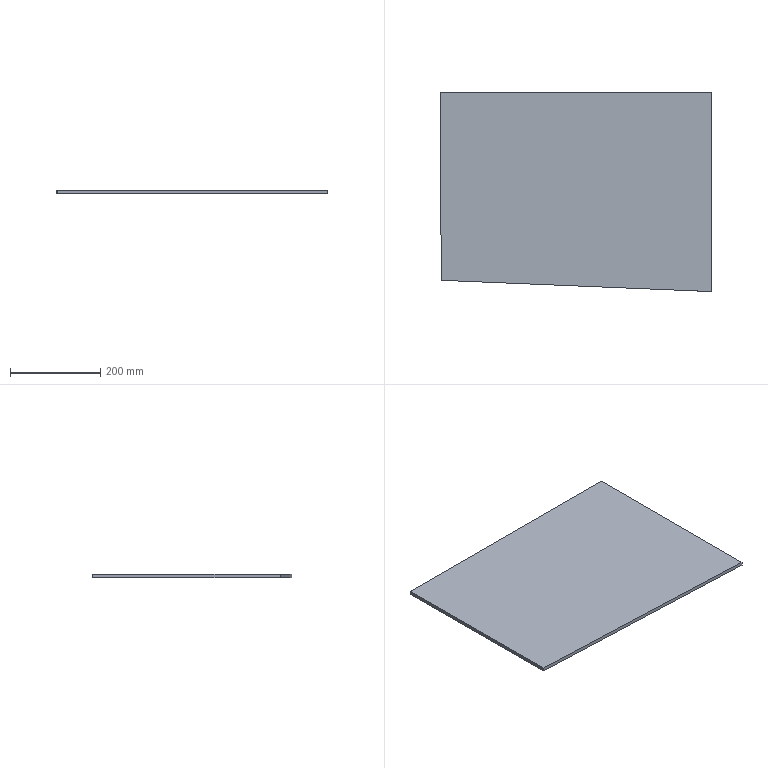Part | STEP file | 06-Middle plate | 1 solid | 6 faces | box 600 x 442 x 8 mm | volume 2060678 mm3 | plane 6
STEP:
#1=CARTESIAN_POINT('',(0.,0.,0.));
#2=DIRECTION('',(0.,0.,1.));
#3=DIRECTION('',(1.,0.,0.));
#4=AXIS2_PLACEMENT_3D('',#1,#2,#3);
#5=CARTESIAN_POINT('',(0.,0.,0.));
#6=VERTEX_POINT('',#5);
#7=CARTESIAN_POINT('',(0.5211,-417.,0.));
#8=VERTEX_POINT('',#7);
#9=CARTESIAN_POINT('',(0.,0.,0.));
#10=DIRECTION('',(0.00125,-1.,0.));
#11=VECTOR('',#10,1.);
#12=LINE('',#9,#11);
#13=CARTESIAN_POINT('',(0.,0.,8.));
#14=DIRECTION('',(1.,0.00125,0.));
#15=DIRECTION('',(-0.00125,1.,0.));
#16=AXIS2_PLACEMENT_3D('',#13,#14,#15);
#17=PLANE('',#16);
#18=CARTESIAN_POINT('',(0.,-8.));
#19=DIRECTION('',(-1.,0.));
#20=VECTOR('',#19,1.);
#21=LINE('',#18,#20);
#22=(GEOMETRIC_REPRESENTATION_CONTEXT(2)PARAMETRIC_REPRESENTATION_CONTEXT()REPRESENTATION_CONTEXT('',''));
#23=DEFINITIONAL_REPRESENTATION('',(#21),#22);
#24=PCURVE('',#17,#23);
#25=CARTESIAN_POINT('',(0.,0.,0.));
#26=DIRECTION('',(0.,0.,1.));
#27=DIRECTION('',(1.,0.,0.));
#28=AXIS2_PLACEMENT_3D('',#25,#26,#27);
#29=PLANE('',#28);
#30=CARTESIAN_POINT('',(0.,0.));
#31=DIRECTION('',(0.00125,-1.));
#32=VECTOR('',#31,1.);
#33=LINE('',#30,#32);
#34=(GEOMETRIC_REPRESENTATION_CONTEXT(2)PARAMETRIC_REPRESENTATION_CONTEXT()REPRESENTATION_CONTEXT('',''));
#35=DEFINITIONAL_REPRESENTATION('',(#33),#34);
#36=PCURVE('',#29,#35);
#37=SURFACE_CURVE('',#12,(#24,#36),.PCURVE_S1.);
#38=EDGE_CURVE('',#6,#8,#37,.T.);
#39=ORIENTED_EDGE('',*,*,#38,.T.);
#40=CARTESIAN_POINT('',(0.5211,-417.,8.));
#41=VERTEX_POINT('',#40);
#42=CARTESIAN_POINT('',(0.5211,-417.,8.));
#43=DIRECTION('',(0.,0.,-1.));
#44=VECTOR('',#43,1.);
#45=LINE('',#42,#44);
#46=CARTESIAN_POINT('',(-417.,0.));
#47=DIRECTION('',(0.,-1.));
#48=VECTOR('',#47,1.);
#49=LINE('',#46,#48);
#50=(GEOMETRIC_REPRESENTATION_CONTEXT(2)PARAMETRIC_REPRESENTATION_CONTEXT()REPRESENTATION_CONTEXT('',''));
#51=DEFINITIONAL_REPRESENTATION('',(#49),#50);
#52=PCURVE('',#17,#51);
#53=CARTESIAN_POINT('',(0.5211,-417.,8.));
#54=DIRECTION('',(0.04167,0.9991,0.));
#55=DIRECTION('',(-0.9991,0.04167,0.));
#56=AXIS2_PLACEMENT_3D('',#53,#54,#55);
#57=PLANE('',#56);
#58=CARTESIAN_POINT('',(0.,0.));
#59=DIRECTION('',(0.,-1.));
#60=VECTOR('',#59,1.);
#61=LINE('',#58,#60);
#62=(GEOMETRIC_REPRESENTATION_CONTEXT(2)PARAMETRIC_REPRESENTATION_CONTEXT()REPRESENTATION_CONTEXT('',''));
#63=DEFINITIONAL_REPRESENTATION('',(#61),#62);
#64=PCURVE('',#57,#63);
#65=SURFACE_CURVE('',#45,(#52,#64),.PCURVE_S1.);
#66=EDGE_CURVE('',#41,#8,#65,.T.);
#67=ORIENTED_EDGE('',*,*,#66,.F.);
#68=CARTESIAN_POINT('',(0.,0.,8.));
#69=VERTEX_POINT('',#68);
#70=CARTESIAN_POINT('',(0.,0.,8.));
#71=DIRECTION('',(0.00125,-1.,0.));
#72=VECTOR('',#71,1.);
#73=LINE('',#70,#72);
#74=CARTESIAN_POINT('',(0.,0.));
#75=DIRECTION('',(-1.,0.));
#76=VECTOR('',#75,1.);
#77=LINE('',#74,#76);
#78=(GEOMETRIC_REPRESENTATION_CONTEXT(2)PARAMETRIC_REPRESENTATION_CONTEXT()REPRESENTATION_CONTEXT('',''));
#79=DEFINITIONAL_REPRESENTATION('',(#77),#78);
#80=PCURVE('',#17,#79);
#81=CARTESIAN_POINT('',(0.,0.,8.));
#82=DIRECTION('',(0.,0.,1.));
#83=DIRECTION('',(1.,0.,0.));
#84=AXIS2_PLACEMENT_3D('',#81,#82,#83);
#85=PLANE('',#84);
#86=CARTESIAN_POINT('',(0.,0.));
#87=DIRECTION('',(0.00125,-1.));
#88=VECTOR('',#87,1.);
#89=LINE('',#86,#88);
#90=(GEOMETRIC_REPRESENTATION_CONTEXT(2)PARAMETRIC_REPRESENTATION_CONTEXT()REPRESENTATION_CONTEXT('',''));
#91=DEFINITIONAL_REPRESENTATION('',(#89),#90);
#92=PCURVE('',#85,#91);
#93=SURFACE_CURVE('',#73,(#80,#92),.PCURVE_S1.);
#94=EDGE_CURVE('',#69,#41,#93,.T.);
#95=ORIENTED_EDGE('',*,*,#94,.F.);
#96=CARTESIAN_POINT('',(0.,0.,8.));
#97=DIRECTION('',(0.,0.,-1.));
#98=VECTOR('',#97,1.);
#99=LINE('',#96,#98);
#100=CARTESIAN_POINT('',(0.,0.));
#101=DIRECTION('',(0.,-1.));
#102=VECTOR('',#101,1.);
#103=LINE('',#100,#102);
#104=(GEOMETRIC_REPRESENTATION_CONTEXT(2)PARAMETRIC_REPRESENTATION_CONTEXT()REPRESENTATION_CONTEXT('',''));
#105=DEFINITIONAL_REPRESENTATION('',(#103),#104);
#106=PCURVE('',#17,#105);
#107=CARTESIAN_POINT('',(0.,0.,8.));
#108=DIRECTION('',(0.,-1.,0.));
#109=DIRECTION('',(0.,0.,-1.));
#110=AXIS2_PLACEMENT_3D('',#107,#108,#109);
#111=PLANE('',#110);
#112=CARTESIAN_POINT('',(0.,0.));
#113=DIRECTION('',(1.,0.));
#114=VECTOR('',#113,1.);
#115=LINE('',#112,#114);
#116=(GEOMETRIC_REPRESENTATION_CONTEXT(2)PARAMETRIC_REPRESENTATION_CONTEXT()REPRESENTATION_CONTEXT('',''));
#117=DEFINITIONAL_REPRESENTATION('',(#115),#116);
#118=PCURVE('',#111,#117);
#119=SURFACE_CURVE('',#99,(#106,#118),.PCURVE_S1.);
#120=EDGE_CURVE('',#69,#6,#119,.T.);
#121=ORIENTED_EDGE('',*,*,#120,.T.);
#122=EDGE_LOOP('',(#39,#67,#95,#121));
#123=FACE_BOUND('',#122,.T.);
#124=ADVANCED_FACE('',(#123),#17,.F.);
#125=CARTESIAN_POINT('',(600.,-442.,0.));
#126=VERTEX_POINT('',#125);
#127=CARTESIAN_POINT('',(0.5211,-417.,0.));
#128=DIRECTION('',(0.9991,-0.04167,0.));
#129=VECTOR('',#128,1.);
#130=LINE('',#127,#129);
#131=CARTESIAN_POINT('',(0.,-8.));
#132=DIRECTION('',(-1.,0.));
#133=VECTOR('',#132,1.);
#134=LINE('',#131,#133);
#135=(GEOMETRIC_REPRESENTATION_CONTEXT(2)PARAMETRIC_REPRESENTATION_CONTEXT()REPRESENTATION_CONTEXT('',''));
#136=DEFINITIONAL_REPRESENTATION('',(#134),#135);
#137=PCURVE('',#57,#136);
#138=CARTESIAN_POINT('',(0.5211,-417.));
#139=DIRECTION('',(0.9991,-0.04167));
#140=VECTOR('',#139,1.);
#141=LINE('',#138,#140);
#142=(GEOMETRIC_REPRESENTATION_CONTEXT(2)PARAMETRIC_REPRESENTATION_CONTEXT()REPRESENTATION_CONTEXT('',''));
#143=DEFINITIONAL_REPRESENTATION('',(#141),#142);
#144=PCURVE('',#29,#143);
#145=SURFACE_CURVE('',#130,(#137,#144),.PCURVE_S1.);
#146=EDGE_CURVE('',#8,#126,#145,.T.);
#147=ORIENTED_EDGE('',*,*,#146,.T.);
#148=CARTESIAN_POINT('',(600.,-442.,8.));
#149=VERTEX_POINT('',#148);
#150=CARTESIAN_POINT('',(600.,-442.,8.));
#151=DIRECTION('',(0.,0.,-1.));
#152=VECTOR('',#151,1.);
#153=LINE('',#150,#152);
#154=CARTESIAN_POINT('',(-600.,0.));
#155=DIRECTION('',(0.,-1.));
#156=VECTOR('',#155,1.);
#157=LINE('',#154,#156);
#158=(GEOMETRIC_REPRESENTATION_CONTEXT(2)PARAMETRIC_REPRESENTATION_CONTEXT()REPRESENTATION_CONTEXT('',''));
#159=DEFINITIONAL_REPRESENTATION('',(#157),#158);
#160=PCURVE('',#57,#159);
#161=CARTESIAN_POINT('',(600.,0.,8.));
#162=DIRECTION('',(-1.,0.,0.));
#163=DIRECTION('',(0.,-1.,0.));
#164=AXIS2_PLACEMENT_3D('',#161,#162,#163);
#165=PLANE('',#164);
#166=CARTESIAN_POINT('',(442.,0.));
#167=DIRECTION('',(0.,-1.));
#168=VECTOR('',#167,1.);
#169=LINE('',#166,#168);
#170=(GEOMETRIC_REPRESENTATION_CONTEXT(2)PARAMETRIC_REPRESENTATION_CONTEXT()REPRESENTATION_CONTEXT('',''));
#171=DEFINITIONAL_REPRESENTATION('',(#169),#170);
#172=PCURVE('',#165,#171);
#173=SURFACE_CURVE('',#153,(#160,#172),.PCURVE_S1.);
#174=EDGE_CURVE('',#149,#126,#173,.T.);
#175=ORIENTED_EDGE('',*,*,#174,.F.);
#176=CARTESIAN_POINT('',(0.5211,-417.,8.));
#177=DIRECTION('',(0.9991,-0.04167,0.));
#178=VECTOR('',#177,1.);
#179=LINE('',#176,#178);
#180=CARTESIAN_POINT('',(0.,0.));
#181=DIRECTION('',(-1.,0.));
#182=VECTOR('',#181,1.);
#183=LINE('',#180,#182);
#184=(GEOMETRIC_REPRESENTATION_CONTEXT(2)PARAMETRIC_REPRESENTATION_CONTEXT()REPRESENTATION_CONTEXT('',''));
#185=DEFINITIONAL_REPRESENTATION('',(#183),#184);
#186=PCURVE('',#57,#185);
#187=CARTESIAN_POINT('',(0.5211,-417.));
#188=DIRECTION('',(0.9991,-0.04167));
#189=VECTOR('',#188,1.);
#190=LINE('',#187,#189);
#191=(GEOMETRIC_REPRESENTATION_CONTEXT(2)PARAMETRIC_REPRESENTATION_CONTEXT()REPRESENTATION_CONTEXT('',''));
#192=DEFINITIONAL_REPRESENTATION('',(#190),#191);
#193=PCURVE('',#85,#192);
#194=SURFACE_CURVE('',#179,(#186,#193),.PCURVE_S1.);
#195=EDGE_CURVE('',#41,#149,#194,.T.);
#196=ORIENTED_EDGE('',*,*,#195,.F.);
#197=ORIENTED_EDGE('',*,*,#66,.T.);
#198=EDGE_LOOP('',(#147,#175,#196,#197));
#199=FACE_BOUND('',#198,.T.);
#200=ADVANCED_FACE('',(#199),#57,.F.);
#201=CARTESIAN_POINT('',(600.,0.,0.));
#202=VERTEX_POINT('',#201);
#203=CARTESIAN_POINT('',(600.,0.,0.));
#204=DIRECTION('',(0.,1.,0.));
#205=VECTOR('',#204,1.);
#206=LINE('',#203,#205);
#207=CARTESIAN_POINT('',(0.,-8.));
#208=DIRECTION('',(-1.,0.));
#209=VECTOR('',#208,1.);
#210=LINE('',#207,#209);
#211=(GEOMETRIC_REPRESENTATION_CONTEXT(2)PARAMETRIC_REPRESENTATION_CONTEXT()REPRESENTATION_CONTEXT('',''));
#212=DEFINITIONAL_REPRESENTATION('',(#210),#211);
#213=PCURVE('',#165,#212);
#214=CARTESIAN_POINT('',(600.,0.));
#215=DIRECTION('',(0.,1.));
#216=VECTOR('',#215,1.);
#217=LINE('',#214,#216);
#218=(GEOMETRIC_REPRESENTATION_CONTEXT(2)PARAMETRIC_REPRESENTATION_CONTEXT()REPRESENTATION_CONTEXT('',''));
#219=DEFINITIONAL_REPRESENTATION('',(#217),#218);
#220=PCURVE('',#29,#219);
#221=SURFACE_CURVE('',#206,(#213,#220),.PCURVE_S1.);
#222=EDGE_CURVE('',#126,#202,#221,.T.);
#223=ORIENTED_EDGE('',*,*,#222,.T.);
#224=CARTESIAN_POINT('',(600.,0.,8.));
#225=VERTEX_POINT('',#224);
#226=CARTESIAN_POINT('',(600.,0.,8.));
#227=DIRECTION('',(0.,0.,-1.));
#228=VECTOR('',#227,1.);
#229=LINE('',#226,#228);
#230=CARTESIAN_POINT('',(0.,0.));
#231=DIRECTION('',(0.,-1.));
#232=VECTOR('',#231,1.);
#233=LINE('',#230,#232);
#234=(GEOMETRIC_REPRESENTATION_CONTEXT(2)PARAMETRIC_REPRESENTATION_CONTEXT()REPRESENTATION_CONTEXT('',''));
#235=DEFINITIONAL_REPRESENTATION('',(#233),#234);
#236=PCURVE('',#165,#235);
#237=CARTESIAN_POINT('',(0.,600.));
#238=DIRECTION('',(1.,0.));
#239=VECTOR('',#238,1.);
#240=LINE('',#237,#239);
#241=(GEOMETRIC_REPRESENTATION_CONTEXT(2)PARAMETRIC_REPRESENTATION_CONTEXT()REPRESENTATION_CONTEXT('',''));
#242=DEFINITIONAL_REPRESENTATION('',(#240),#241);
#243=PCURVE('',#111,#242);
#244=SURFACE_CURVE('',#229,(#236,#243),.PCURVE_S1.);
#245=EDGE_CURVE('',#225,#202,#244,.T.);
#246=ORIENTED_EDGE('',*,*,#245,.F.);
#247=CARTESIAN_POINT('',(600.,0.,8.));
#248=DIRECTION('',(0.,1.,0.));
#249=VECTOR('',#248,1.);
#250=LINE('',#247,#249);
#251=CARTESIAN_POINT('',(0.,0.));
#252=DIRECTION('',(-1.,0.));
#253=VECTOR('',#252,1.);
#254=LINE('',#251,#253);
#255=(GEOMETRIC_REPRESENTATION_CONTEXT(2)PARAMETRIC_REPRESENTATION_CONTEXT()REPRESENTATION_CONTEXT('',''));
#256=DEFINITIONAL_REPRESENTATION('',(#254),#255);
#257=PCURVE('',#165,#256);
#258=CARTESIAN_POINT('',(600.,0.));
#259=DIRECTION('',(0.,1.));
#260=VECTOR('',#259,1.);
#261=LINE('',#258,#260);
#262=(GEOMETRIC_REPRESENTATION_CONTEXT(2)PARAMETRIC_REPRESENTATION_CONTEXT()REPRESENTATION_CONTEXT('',''));
#263=DEFINITIONAL_REPRESENTATION('',(#261),#262);
#264=PCURVE('',#85,#263);
#265=SURFACE_CURVE('',#250,(#257,#264),.PCURVE_S1.);
#266=EDGE_CURVE('',#149,#225,#265,.T.);
#267=ORIENTED_EDGE('',*,*,#266,.F.);
#268=ORIENTED_EDGE('',*,*,#174,.T.);
#269=EDGE_LOOP('',(#223,#246,#267,#268));
#270=FACE_BOUND('',#269,.T.);
#271=ADVANCED_FACE('',(#270),#165,.F.);
#272=CARTESIAN_POINT('',(0.,0.,0.));
#273=DIRECTION('',(-1.,0.,0.));
#274=VECTOR('',#273,1.);
#275=LINE('',#272,#274);
#276=CARTESIAN_POINT('',(8.,0.));
#277=DIRECTION('',(0.,-1.));
#278=VECTOR('',#277,1.);
#279=LINE('',#276,#278);
#280=(GEOMETRIC_REPRESENTATION_CONTEXT(2)PARAMETRIC_REPRESENTATION_CONTEXT()REPRESENTATION_CONTEXT('',''));
#281=DEFINITIONAL_REPRESENTATION('',(#279),#280);
#282=PCURVE('',#111,#281);
#283=CARTESIAN_POINT('',(0.,0.));
#284=DIRECTION('',(-1.,0.));
#285=VECTOR('',#284,1.);
#286=LINE('',#283,#285);
#287=(GEOMETRIC_REPRESENTATION_CONTEXT(2)PARAMETRIC_REPRESENTATION_CONTEXT()REPRESENTATION_CONTEXT('',''));
#288=DEFINITIONAL_REPRESENTATION('',(#286),#287);
#289=PCURVE('',#29,#288);
#290=SURFACE_CURVE('',#275,(#282,#289),.PCURVE_S1.);
#291=EDGE_CURVE('',#202,#6,#290,.T.);
#292=ORIENTED_EDGE('',*,*,#291,.T.);
#293=ORIENTED_EDGE('',*,*,#120,.F.);
#294=CARTESIAN_POINT('',(0.,0.,8.));
#295=DIRECTION('',(-1.,0.,0.));
#296=VECTOR('',#295,1.);
#297=LINE('',#294,#296);
#298=CARTESIAN_POINT('',(0.,0.));
#299=DIRECTION('',(0.,-1.));
#300=VECTOR('',#299,1.);
#301=LINE('',#298,#300);
#302=(GEOMETRIC_REPRESENTATION_CONTEXT(2)PARAMETRIC_REPRESENTATION_CONTEXT()REPRESENTATION_CONTEXT('',''));
#303=DEFINITIONAL_REPRESENTATION('',(#301),#302);
#304=PCURVE('',#111,#303);
#305=CARTESIAN_POINT('',(0.,0.));
#306=DIRECTION('',(-1.,0.));
#307=VECTOR('',#306,1.);
#308=LINE('',#305,#307);
#309=(GEOMETRIC_REPRESENTATION_CONTEXT(2)PARAMETRIC_REPRESENTATION_CONTEXT()REPRESENTATION_CONTEXT('',''));
#310=DEFINITIONAL_REPRESENTATION('',(#308),#309);
#311=PCURVE('',#85,#310);
#312=SURFACE_CURVE('',#297,(#304,#311),.PCURVE_S1.);
#313=EDGE_CURVE('',#225,#69,#312,.T.);
#314=ORIENTED_EDGE('',*,*,#313,.F.);
#315=ORIENTED_EDGE('',*,*,#245,.T.);
#316=EDGE_LOOP('',(#292,#293,#314,#315));
#317=FACE_BOUND('',#316,.T.);
#318=ADVANCED_FACE('',(#317),#111,.F.);
#319=ORIENTED_EDGE('',*,*,#94,.T.);
#320=ORIENTED_EDGE('',*,*,#195,.T.);
#321=ORIENTED_EDGE('',*,*,#266,.T.);
#322=ORIENTED_EDGE('',*,*,#313,.T.);
#323=EDGE_LOOP('',(#319,#320,#321,#322));
#324=FACE_BOUND('',#323,.T.);
#325=ADVANCED_FACE('',(#324),#85,.T.);
#326=ORIENTED_EDGE('',*,*,#38,.F.);
#327=ORIENTED_EDGE('',*,*,#291,.F.);
#328=ORIENTED_EDGE('',*,*,#222,.F.);
#329=ORIENTED_EDGE('',*,*,#146,.F.);
#330=EDGE_LOOP('',(#326,#327,#328,#329));
#331=FACE_BOUND('',#330,.T.);
#332=ADVANCED_FACE('',(#331),#29,.F.);
#333=CLOSED_SHELL('',(#124,#200,#271,#318,#325,#332));
#334=MANIFOLD_SOLID_BREP('',#333);
#335=(LENGTH_UNIT()NAMED_UNIT(*)SI_UNIT(.MILLI.,.METRE.));
#336=UNCERTAINTY_MEASURE_WITH_UNIT(LENGTH_MEASURE(0.0000001),#335,'','');
#337=(NAMED_UNIT(*)PLANE_ANGLE_UNIT()SI_UNIT($,.RADIAN.));
#338=(NAMED_UNIT(*)SI_UNIT($,.STERADIAN.)SOLID_ANGLE_UNIT());
#339=(GEOMETRIC_REPRESENTATION_CONTEXT(3)GLOBAL_UNCERTAINTY_ASSIGNED_CONTEXT((#336))GLOBAL_UNIT_ASSIGNED_CONTEXT((#335,#337,#338))REPRESENTATION_CONTEXT('',''));
#340=ADVANCED_BREP_SHAPE_REPRESENTATION('',(#4,#334),#339);